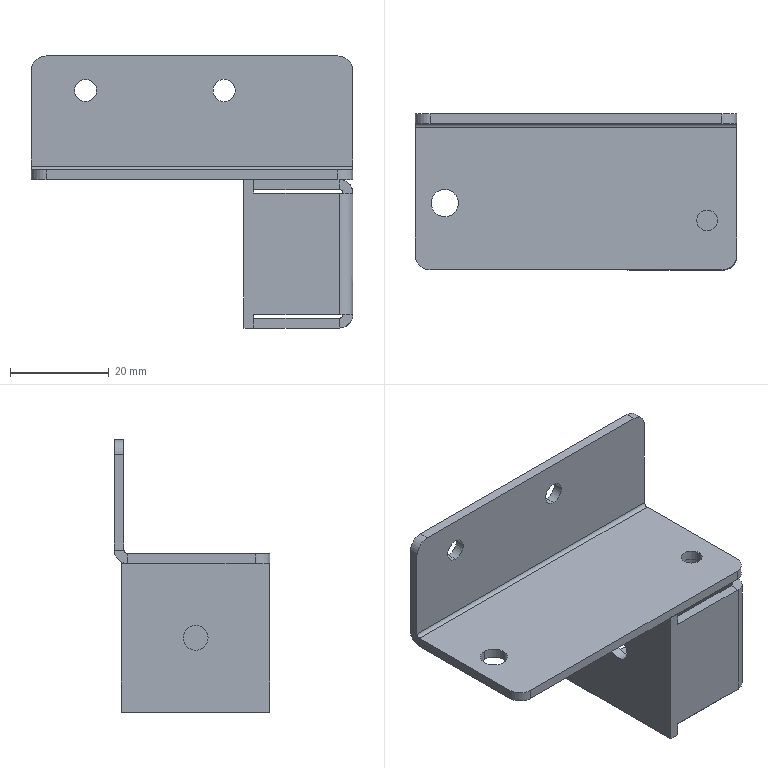Part | SolidWorks | features HoleWzd 4, EdgeFlange 2, FlatPattern 2, ICE 2, SMBaseFlange 2, SheetMetal 2, Fillet 1 | 2 solids | 68 faces | box 65 x 31.5 x 55 mm | volume 13652 mm3 | plane 32 | cylinder 28 | spline 8 | commonest cylinder face diameters 5.5 x9 1.5 x5 4.2 x4 4.5 x4 6 x4 5 x2